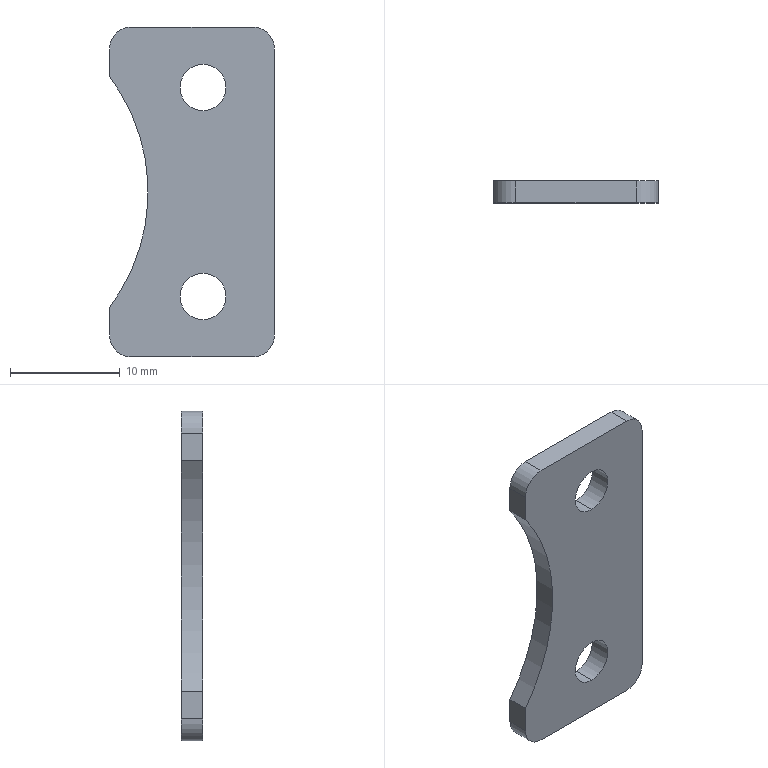Part | STEP file | 1 solid | 16 faces | box 15 x 2 x 30 mm | volume 737.571 mm3 | cylinder 9 | plane 7 | commonest cylinder face diameters 4 x4 4.2 x4 35 x1
STEP:
#1=CARTESIAN_POINT('',(0.,0.,0.));
#2=DIRECTION('',(0.,0.,1.));
#3=DIRECTION('',(1.,0.,0.));
#4=AXIS2_PLACEMENT_3D('',#1,#2,#3);
#5=CARTESIAN_POINT('',(1.,2.,7.4));
#6=VERTEX_POINT('',#5);
#7=CARTESIAN_POINT('',(1.,0.,7.4));
#8=VERTEX_POINT('',#7);
#9=CARTESIAN_POINT('',(1.,0.,7.4));
#10=DIRECTION('',(0.,-1.,0.));
#11=VECTOR('',#10,1.);
#12=LINE('',#9,#11);
#13=CARTESIAN_POINT('',(1.,0.,9.5));
#14=DIRECTION('',(0.,-1.,0.));
#15=DIRECTION('',(0.,0.,-1.));
#16=AXIS2_PLACEMENT_3D('',#13,#14,#15);
#17=CYLINDRICAL_SURFACE('',#16,2.1);
#18=CARTESIAN_POINT('',(6.283,0.));
#19=DIRECTION('',(0.,1.));
#20=VECTOR('',#19,1.);
#21=LINE('',#18,#20);
#22=(GEOMETRIC_REPRESENTATION_CONTEXT(2)PARAMETRIC_REPRESENTATION_CONTEXT()REPRESENTATION_CONTEXT('',''));
#23=DEFINITIONAL_REPRESENTATION('',(#21),#22);
#24=PCURVE('',#17,#23);
#25=CARTESIAN_POINT('',(1.,0.,9.5));
#26=DIRECTION('',(0.,-1.,0.));
#27=DIRECTION('',(0.,0.,-1.));
#28=AXIS2_PLACEMENT_3D('',#25,#26,#27);
#29=CYLINDRICAL_SURFACE('',#28,2.1);
#30=CARTESIAN_POINT('',(0.,0.));
#31=DIRECTION('',(0.,1.));
#32=VECTOR('',#31,1.);
#33=LINE('',#30,#32);
#34=(GEOMETRIC_REPRESENTATION_CONTEXT(2)PARAMETRIC_REPRESENTATION_CONTEXT()REPRESENTATION_CONTEXT('',''));
#35=DEFINITIONAL_REPRESENTATION('',(#33),#34);
#36=PCURVE('',#29,#35);
#37=SURFACE_CURVE('',#12,(#24,#36),.PCURVE_S1.);
#38=EDGE_CURVE('',#6,#8,#37,.T.);
#39=ORIENTED_EDGE('',*,*,#38,.T.);
#40=CARTESIAN_POINT('',(1.,0.,11.6));
#41=VERTEX_POINT('',#40);
#42=CARTESIAN_POINT('',(1.,0.,9.5));
#43=DIRECTION('',(0.,-1.,0.));
#44=DIRECTION('',(0.,0.,-1.));
#45=AXIS2_PLACEMENT_3D('',#42,#43,#44);
#46=CIRCLE('',#45,2.1);
#47=CARTESIAN_POINT('',(0.,0.));
#48=DIRECTION('',(1.,0.));
#49=VECTOR('',#48,1.);
#50=LINE('',#47,#49);
#51=(GEOMETRIC_REPRESENTATION_CONTEXT(2)PARAMETRIC_REPRESENTATION_CONTEXT()REPRESENTATION_CONTEXT('',''));
#52=DEFINITIONAL_REPRESENTATION('',(#50),#51);
#53=PCURVE('',#17,#52);
#54=CARTESIAN_POINT('',(0.,0.,0.));
#55=DIRECTION('',(0.,1.,0.));
#56=DIRECTION('',(0.,0.,1.));
#57=AXIS2_PLACEMENT_3D('',#54,#55,#56);
#58=PLANE('',#57);
#59=CARTESIAN_POINT('',(7.4,1.));
#60=CARTESIAN_POINT('',(7.4,4.637));
#61=CARTESIAN_POINT('',(10.55,2.819));
#62=CARTESIAN_POINT('',(13.7,1.));
#63=CARTESIAN_POINT('',(10.55,-0.8187));
#64=CARTESIAN_POINT('',(7.4,-2.637));
#65=CARTESIAN_POINT('',(7.4,1.));
#66=(BOUNDED_CURVE()B_SPLINE_CURVE(2,(#59,#60,#61,#62,#63,#64,#65),.UNSPECIFIED.,.T.,.F.)B_SPLINE_CURVE_WITH_KNOTS((1,2,2,2,2,1),(-2.094,0.,2.094,4.189,6.283,8.378),.UNSPECIFIED.)CURVE()GEOMETRIC_REPRESENTATION_ITEM()RATIONAL_B_SPLINE_CURVE((1.,0.5,1.,0.5,1.,0.5,1.))REPRESENTATION_ITEM(''));
#67=(GEOMETRIC_REPRESENTATION_CONTEXT(2)PARAMETRIC_REPRESENTATION_CONTEXT()REPRESENTATION_CONTEXT('',''));
#68=DEFINITIONAL_REPRESENTATION('',(#66),#67);
#69=PCURVE('',#58,#68);
#70=SURFACE_CURVE('',#46,(#53,#69),.PCURVE_S1.);
#71=EDGE_CURVE('',#41,#8,#70,.T.);
#72=ORIENTED_EDGE('',*,*,#71,.F.);
#73=CARTESIAN_POINT('',(1.,2.,11.6));
#74=VERTEX_POINT('',#73);
#75=CARTESIAN_POINT('',(1.,0.,11.6));
#76=DIRECTION('',(0.,-1.,0.));
#77=VECTOR('',#76,1.);
#78=LINE('',#75,#77);
#79=CARTESIAN_POINT('',(3.142,0.));
#80=DIRECTION('',(0.,1.));
#81=VECTOR('',#80,1.);
#82=LINE('',#79,#81);
#83=(GEOMETRIC_REPRESENTATION_CONTEXT(2)PARAMETRIC_REPRESENTATION_CONTEXT()REPRESENTATION_CONTEXT('',''));
#84=DEFINITIONAL_REPRESENTATION('',(#82),#83);
#85=PCURVE('',#17,#84);
#86=CARTESIAN_POINT('',(3.142,0.));
#87=DIRECTION('',(0.,1.));
#88=VECTOR('',#87,1.);
#89=LINE('',#86,#88);
#90=(GEOMETRIC_REPRESENTATION_CONTEXT(2)PARAMETRIC_REPRESENTATION_CONTEXT()REPRESENTATION_CONTEXT('',''));
#91=DEFINITIONAL_REPRESENTATION('',(#89),#90);
#92=PCURVE('',#29,#91);
#93=SURFACE_CURVE('',#78,(#85,#92),.PCURVE_S1.);
#94=EDGE_CURVE('',#74,#41,#93,.T.);
#95=ORIENTED_EDGE('',*,*,#94,.F.);
#96=CARTESIAN_POINT('',(1.,2.,9.5));
#97=DIRECTION('',(0.,-1.,0.));
#98=DIRECTION('',(0.,0.,-1.));
#99=AXIS2_PLACEMENT_3D('',#96,#97,#98);
#100=CIRCLE('',#99,2.1);
#101=CARTESIAN_POINT('',(0.,-2.));
#102=DIRECTION('',(1.,0.));
#103=VECTOR('',#102,1.);
#104=LINE('',#101,#103);
#105=(GEOMETRIC_REPRESENTATION_CONTEXT(2)PARAMETRIC_REPRESENTATION_CONTEXT()REPRESENTATION_CONTEXT('',''));
#106=DEFINITIONAL_REPRESENTATION('',(#104),#105);
#107=PCURVE('',#17,#106);
#108=CARTESIAN_POINT('',(0.,2.,0.));
#109=DIRECTION('',(0.,1.,0.));
#110=DIRECTION('',(0.,0.,1.));
#111=AXIS2_PLACEMENT_3D('',#108,#109,#110);
#112=PLANE('',#111);
#113=CARTESIAN_POINT('',(7.4,1.));
#114=CARTESIAN_POINT('',(7.4,4.637));
#115=CARTESIAN_POINT('',(10.55,2.819));
#116=CARTESIAN_POINT('',(13.7,1.));
#117=CARTESIAN_POINT('',(10.55,-0.8187));
#118=CARTESIAN_POINT('',(7.4,-2.637));
#119=CARTESIAN_POINT('',(7.4,1.));
#120=(BOUNDED_CURVE()B_SPLINE_CURVE(2,(#113,#114,#115,#116,#117,#118,#119),.UNSPECIFIED.,.T.,.F.)B_SPLINE_CURVE_WITH_KNOTS((1,2,2,2,2,1),(-2.094,0.,2.094,4.189,6.283,8.378),.UNSPECIFIED.)CURVE()GEOMETRIC_REPRESENTATION_ITEM()RATIONAL_B_SPLINE_CURVE((1.,0.5,1.,0.5,1.,0.5,1.))REPRESENTATION_ITEM(''));
#121=(GEOMETRIC_REPRESENTATION_CONTEXT(2)PARAMETRIC_REPRESENTATION_CONTEXT()REPRESENTATION_CONTEXT('',''));
#122=DEFINITIONAL_REPRESENTATION('',(#120),#121);
#123=PCURVE('',#112,#122);
#124=SURFACE_CURVE('',#100,(#107,#123),.PCURVE_S1.);
#125=EDGE_CURVE('',#74,#6,#124,.T.);
#126=ORIENTED_EDGE('',*,*,#125,.T.);
#127=EDGE_LOOP('',(#39,#72,#95,#126));
#128=FACE_BOUND('',#127,.F.);
#129=ADVANCED_FACE('',(#128),#17,.F.);
#130=CARTESIAN_POINT('',(1.,2.,-11.6));
#131=VERTEX_POINT('',#130);
#132=CARTESIAN_POINT('',(1.,0.,-11.6));
#133=VERTEX_POINT('',#132);
#134=CARTESIAN_POINT('',(1.,0.,-11.6));
#135=DIRECTION('',(0.,-1.,0.));
#136=VECTOR('',#135,1.);
#137=LINE('',#134,#136);
#138=CARTESIAN_POINT('',(1.,0.,-9.5));
#139=DIRECTION('',(0.,-1.,0.));
#140=DIRECTION('',(0.,0.,-1.));
#141=AXIS2_PLACEMENT_3D('',#138,#139,#140);
#142=CYLINDRICAL_SURFACE('',#141,2.1);
#143=CARTESIAN_POINT('',(6.283,0.));
#144=DIRECTION('',(0.,1.));
#145=VECTOR('',#144,1.);
#146=LINE('',#143,#145);
#147=(GEOMETRIC_REPRESENTATION_CONTEXT(2)PARAMETRIC_REPRESENTATION_CONTEXT()REPRESENTATION_CONTEXT('',''));
#148=DEFINITIONAL_REPRESENTATION('',(#146),#147);
#149=PCURVE('',#142,#148);
#150=CARTESIAN_POINT('',(1.,0.,-9.5));
#151=DIRECTION('',(0.,-1.,0.));
#152=DIRECTION('',(0.,0.,-1.));
#153=AXIS2_PLACEMENT_3D('',#150,#151,#152);
#154=CYLINDRICAL_SURFACE('',#153,2.1);
#155=CARTESIAN_POINT('',(0.,0.));
#156=DIRECTION('',(0.,1.));
#157=VECTOR('',#156,1.);
#158=LINE('',#155,#157);
#159=(GEOMETRIC_REPRESENTATION_CONTEXT(2)PARAMETRIC_REPRESENTATION_CONTEXT()REPRESENTATION_CONTEXT('',''));
#160=DEFINITIONAL_REPRESENTATION('',(#158),#159);
#161=PCURVE('',#154,#160);
#162=SURFACE_CURVE('',#137,(#149,#161),.PCURVE_S1.);
#163=EDGE_CURVE('',#131,#133,#162,.T.);
#164=ORIENTED_EDGE('',*,*,#163,.T.);
#165=CARTESIAN_POINT('',(1.,0.,-7.4));
#166=VERTEX_POINT('',#165);
#167=CARTESIAN_POINT('',(1.,0.,-9.5));
#168=DIRECTION('',(0.,-1.,0.));
#169=DIRECTION('',(0.,0.,-1.));
#170=AXIS2_PLACEMENT_3D('',#167,#168,#169);
#171=CIRCLE('',#170,2.1);
#172=CARTESIAN_POINT('',(0.,0.));
#173=DIRECTION('',(1.,0.));
#174=VECTOR('',#173,1.);
#175=LINE('',#172,#174);
#176=(GEOMETRIC_REPRESENTATION_CONTEXT(2)PARAMETRIC_REPRESENTATION_CONTEXT()REPRESENTATION_CONTEXT('',''));
#177=DEFINITIONAL_REPRESENTATION('',(#175),#176);
#178=PCURVE('',#142,#177);
#179=CARTESIAN_POINT('',(-11.6,1.));
#180=CARTESIAN_POINT('',(-11.6,4.637));
#181=CARTESIAN_POINT('',(-8.45,2.819));
#182=CARTESIAN_POINT('',(-5.3,1.));
#183=CARTESIAN_POINT('',(-8.45,-0.8187));
#184=CARTESIAN_POINT('',(-11.6,-2.637));
#185=CARTESIAN_POINT('',(-11.6,1.));
#186=(BOUNDED_CURVE()B_SPLINE_CURVE(2,(#179,#180,#181,#182,#183,#184,#185),.UNSPECIFIED.,.T.,.F.)B_SPLINE_CURVE_WITH_KNOTS((1,2,2,2,2,1),(-2.094,0.,2.094,4.189,6.283,8.378),.UNSPECIFIED.)CURVE()GEOMETRIC_REPRESENTATION_ITEM()RATIONAL_B_SPLINE_CURVE((1.,0.5,1.,0.5,1.,0.5,1.))REPRESENTATION_ITEM(''));
#187=(GEOMETRIC_REPRESENTATION_CONTEXT(2)PARAMETRIC_REPRESENTATION_CONTEXT()REPRESENTATION_CONTEXT('',''));
#188=DEFINITIONAL_REPRESENTATION('',(#186),#187);
#189=PCURVE('',#58,#188);
#190=SURFACE_CURVE('',#171,(#178,#189),.PCURVE_S1.);
#191=EDGE_CURVE('',#166,#133,#190,.T.);
#192=ORIENTED_EDGE('',*,*,#191,.F.);
#193=CARTESIAN_POINT('',(1.,2.,-7.4));
#194=VERTEX_POINT('',#193);
#195=CARTESIAN_POINT('',(1.,0.,-7.4));
#196=DIRECTION('',(0.,-1.,0.));
#197=VECTOR('',#196,1.);
#198=LINE('',#195,#197);
#199=CARTESIAN_POINT('',(3.142,0.));
#200=DIRECTION('',(0.,1.));
#201=VECTOR('',#200,1.);
#202=LINE('',#199,#201);
#203=(GEOMETRIC_REPRESENTATION_CONTEXT(2)PARAMETRIC_REPRESENTATION_CONTEXT()REPRESENTATION_CONTEXT('',''));
#204=DEFINITIONAL_REPRESENTATION('',(#202),#203);
#205=PCURVE('',#142,#204);
#206=CARTESIAN_POINT('',(3.142,0.));
#207=DIRECTION('',(0.,1.));
#208=VECTOR('',#207,1.);
#209=LINE('',#206,#208);
#210=(GEOMETRIC_REPRESENTATION_CONTEXT(2)PARAMETRIC_REPRESENTATION_CONTEXT()REPRESENTATION_CONTEXT('',''));
#211=DEFINITIONAL_REPRESENTATION('',(#209),#210);
#212=PCURVE('',#154,#211);
#213=SURFACE_CURVE('',#198,(#205,#212),.PCURVE_S1.);
#214=EDGE_CURVE('',#194,#166,#213,.T.);
#215=ORIENTED_EDGE('',*,*,#214,.F.);
#216=CARTESIAN_POINT('',(1.,2.,-9.5));
#217=DIRECTION('',(0.,-1.,0.));
#218=DIRECTION('',(0.,0.,-1.));
#219=AXIS2_PLACEMENT_3D('',#216,#217,#218);
#220=CIRCLE('',#219,2.1);
#221=CARTESIAN_POINT('',(0.,-2.));
#222=DIRECTION('',(1.,0.));
#223=VECTOR('',#222,1.);
#224=LINE('',#221,#223);
#225=(GEOMETRIC_REPRESENTATION_CONTEXT(2)PARAMETRIC_REPRESENTATION_CONTEXT()REPRESENTATION_CONTEXT('',''));
#226=DEFINITIONAL_REPRESENTATION('',(#224),#225);
#227=PCURVE('',#142,#226);
#228=CARTESIAN_POINT('',(-11.6,1.));
#229=CARTESIAN_POINT('',(-11.6,4.637));
#230=CARTESIAN_POINT('',(-8.45,2.819));
#231=CARTESIAN_POINT('',(-5.3,1.));
#232=CARTESIAN_POINT('',(-8.45,-0.8187));
#233=CARTESIAN_POINT('',(-11.6,-2.637));
#234=CARTESIAN_POINT('',(-11.6,1.));
#235=(BOUNDED_CURVE()B_SPLINE_CURVE(2,(#228,#229,#230,#231,#232,#233,#234),.UNSPECIFIED.,.T.,.F.)B_SPLINE_CURVE_WITH_KNOTS((1,2,2,2,2,1),(-2.094,0.,2.094,4.189,6.283,8.378),.UNSPECIFIED.)CURVE()GEOMETRIC_REPRESENTATION_ITEM()RATIONAL_B_SPLINE_CURVE((1.,0.5,1.,0.5,1.,0.5,1.))REPRESENTATION_ITEM(''));
#236=(GEOMETRIC_REPRESENTATION_CONTEXT(2)PARAMETRIC_REPRESENTATION_CONTEXT()REPRESENTATION_CONTEXT('',''));
#237=DEFINITIONAL_REPRESENTATION('',(#235),#236);
#238=PCURVE('',#112,#237);
#239=SURFACE_CURVE('',#220,(#227,#238),.PCURVE_S1.);
#240=EDGE_CURVE('',#194,#131,#239,.T.);
#241=ORIENTED_EDGE('',*,*,#240,.T.);
#242=EDGE_LOOP('',(#164,#192,#215,#241));
#243=FACE_BOUND('',#242,.F.);
#244=ADVANCED_FACE('',(#243),#142,.F.);
#245=CARTESIAN_POINT('',(-7.5,2.,-13.));
#246=VERTEX_POINT('',#245);
#247=CARTESIAN_POINT('',(-7.5,2.,-10.5));
#248=VERTEX_POINT('',#247);
#249=CARTESIAN_POINT('',(-7.5,2.,15.));
#250=DIRECTION('',(0.,0.,1.));
#251=VECTOR('',#250,1.);
#252=LINE('',#249,#251);
#253=CARTESIAN_POINT('',(-7.5,2.,15.));
#254=DIRECTION('',(1.,0.,0.));
#255=DIRECTION('',(0.,0.,-1.));
#256=AXIS2_PLACEMENT_3D('',#253,#254,#255);
#257=PLANE('',#256);
#258=CARTESIAN_POINT('',(0.,0.));
#259=DIRECTION('',(-1.,0.));
#260=VECTOR('',#259,1.);
#261=LINE('',#258,#260);
#262=(GEOMETRIC_REPRESENTATION_CONTEXT(2)PARAMETRIC_REPRESENTATION_CONTEXT()REPRESENTATION_CONTEXT('',''));
#263=DEFINITIONAL_REPRESENTATION('',(#261),#262);
#264=PCURVE('',#257,#263);
#265=CARTESIAN_POINT('',(15.,-7.5));
#266=DIRECTION('',(1.,0.));
#267=VECTOR('',#266,1.);
#268=LINE('',#265,#267);
#269=(GEOMETRIC_REPRESENTATION_CONTEXT(2)PARAMETRIC_REPRESENTATION_CONTEXT()REPRESENTATION_CONTEXT('',''));
#270=DEFINITIONAL_REPRESENTATION('',(#268),#269);
#271=PCURVE('',#112,#270);
#272=SURFACE_CURVE('',#252,(#264,#271),.PCURVE_S1.);
#273=EDGE_CURVE('',#246,#248,#272,.T.);
#274=ORIENTED_EDGE('',*,*,#273,.F.);
#275=CARTESIAN_POINT('',(-7.5,0.,-13.));
#276=VERTEX_POINT('',#275);
#277=CARTESIAN_POINT('',(-7.5,2.,-13.));
#278=DIRECTION('',(0.,-1.,0.));
#279=VECTOR('',#278,1.);
#280=LINE('',#277,#279);
#281=CARTESIAN_POINT('',(28.,0.));
#282=DIRECTION('',(0.,-1.));
#283=VECTOR('',#282,1.);
#284=LINE('',#281,#283);
#285=(GEOMETRIC_REPRESENTATION_CONTEXT(2)PARAMETRIC_REPRESENTATION_CONTEXT()REPRESENTATION_CONTEXT('',''));
#286=DEFINITIONAL_REPRESENTATION('',(#284),#285);
#287=PCURVE('',#257,#286);
#288=CARTESIAN_POINT('',(-5.5,2.,-13.));
#289=DIRECTION('',(0.,-1.,0.));
#290=DIRECTION('',(0.,0.,-1.));
#291=AXIS2_PLACEMENT_3D('',#288,#289,#290);
#292=CYLINDRICAL_SURFACE('',#291,2.);
#293=CARTESIAN_POINT('',(4.712,0.));
#294=DIRECTION('',(0.,1.));
#295=VECTOR('',#294,1.);
#296=LINE('',#293,#295);
#297=(GEOMETRIC_REPRESENTATION_CONTEXT(2)PARAMETRIC_REPRESENTATION_CONTEXT()REPRESENTATION_CONTEXT('',''));
#298=DEFINITIONAL_REPRESENTATION('',(#296),#297);
#299=PCURVE('',#292,#298);
#300=SURFACE_CURVE('',#280,(#287,#299),.PCURVE_S1.);
#301=EDGE_CURVE('',#246,#276,#300,.T.);
#302=ORIENTED_EDGE('',*,*,#301,.T.);
#303=CARTESIAN_POINT('',(-7.5,0.,-10.5));
#304=VERTEX_POINT('',#303);
#305=CARTESIAN_POINT('',(-7.5,0.,15.));
#306=DIRECTION('',(0.,0.,1.));
#307=VECTOR('',#306,1.);
#308=LINE('',#305,#307);
#309=CARTESIAN_POINT('',(0.,-2.));
#310=DIRECTION('',(-1.,0.));
#311=VECTOR('',#310,1.);
#312=LINE('',#309,#311);
#313=(GEOMETRIC_REPRESENTATION_CONTEXT(2)PARAMETRIC_REPRESENTATION_CONTEXT()REPRESENTATION_CONTEXT('',''));
#314=DEFINITIONAL_REPRESENTATION('',(#312),#313);
#315=PCURVE('',#257,#314);
#316=CARTESIAN_POINT('',(15.,-7.5));
#317=DIRECTION('',(1.,0.));
#318=VECTOR('',#317,1.);
#319=LINE('',#316,#318);
#320=(GEOMETRIC_REPRESENTATION_CONTEXT(2)PARAMETRIC_REPRESENTATION_CONTEXT()REPRESENTATION_CONTEXT('',''));
#321=DEFINITIONAL_REPRESENTATION('',(#319),#320);
#322=PCURVE('',#58,#321);
#323=SURFACE_CURVE('',#308,(#315,#322),.PCURVE_S1.);
#324=EDGE_CURVE('',#276,#304,#323,.T.);
#325=ORIENTED_EDGE('',*,*,#324,.T.);
#326=CARTESIAN_POINT('',(-7.5,0.,-10.5));
#327=DIRECTION('',(0.,1.,0.));
#328=VECTOR('',#327,1.);
#329=LINE('',#326,#328);
#330=CARTESIAN_POINT('',(25.5,-2.));
#331=DIRECTION('',(0.,1.));
#332=VECTOR('',#331,1.);
#333=LINE('',#330,#332);
#334=(GEOMETRIC_REPRESENTATION_CONTEXT(2)PARAMETRIC_REPRESENTATION_CONTEXT()REPRESENTATION_CONTEXT('',''));
#335=DEFINITIONAL_REPRESENTATION('',(#333),#334);
#336=PCURVE('',#257,#335);
#337=CARTESIAN_POINT('',(-21.5,0.,0.));
#338=DIRECTION('',(0.,1.,0.));
#339=DIRECTION('',(0.,0.,1.));
#340=AXIS2_PLACEMENT_3D('',#337,#338,#339);
#341=CYLINDRICAL_SURFACE('',#340,17.5);
#342=CARTESIAN_POINT('',(2.214,0.));
#343=DIRECTION('',(0.,1.));
#344=VECTOR('',#343,1.);
#345=LINE('',#342,#344);
#346=(GEOMETRIC_REPRESENTATION_CONTEXT(2)PARAMETRIC_REPRESENTATION_CONTEXT()REPRESENTATION_CONTEXT('',''));
#347=DEFINITIONAL_REPRESENTATION('',(#345),#346);
#348=PCURVE('',#341,#347);
#349=SURFACE_CURVE('',#329,(#336,#348),.PCURVE_S1.);
#350=EDGE_CURVE('',#304,#248,#349,.T.);
#351=ORIENTED_EDGE('',*,*,#350,.T.);
#352=EDGE_LOOP('',(#274,#302,#325,#351));
#353=FACE_BOUND('',#352,.T.);
#354=ADVANCED_FACE('',(#353),#257,.F.);
#355=CARTESIAN_POINT('',(-7.5,0.,10.5));
#356=VERTEX_POINT('',#355);
#357=CARTESIAN_POINT('',(-7.5,0.,13.));
#358=VERTEX_POINT('',#357);
#359=CARTESIAN_POINT('',(-7.5,0.,15.));
#360=DIRECTION('',(0.,0.,1.));
#361=VECTOR('',#360,1.);
#362=LINE('',#359,#361);
#363=CARTESIAN_POINT('',(-7.5,2.,15.));
#364=DIRECTION('',(1.,0.,0.));
#365=DIRECTION('',(0.,0.,-1.));
#366=AXIS2_PLACEMENT_3D('',#363,#364,#365);
#367=PLANE('',#366);
#368=CARTESIAN_POINT('',(0.,-2.));
#369=DIRECTION('',(-1.,0.));
#370=VECTOR('',#369,1.);
#371=LINE('',#368,#370);
#372=(GEOMETRIC_REPRESENTATION_CONTEXT(2)PARAMETRIC_REPRESENTATION_CONTEXT()REPRESENTATION_CONTEXT('',''));
#373=DEFINITIONAL_REPRESENTATION('',(#371),#372);
#374=PCURVE('',#367,#373);
#375=CARTESIAN_POINT('',(15.,-7.5));
#376=DIRECTION('',(1.,0.));
#377=VECTOR('',#376,1.);
#378=LINE('',#375,#377);
#379=(GEOMETRIC_REPRESENTATION_CONTEXT(2)PARAMETRIC_REPRESENTATION_CONTEXT()REPRESENTATION_CONTEXT('',''));
#380=DEFINITIONAL_REPRESENTATION('',(#378),#379);
#381=PCURVE('',#58,#380);
#382=SURFACE_CURVE('',#362,(#374,#381),.PCURVE_S1.);
#383=EDGE_CURVE('',#356,#358,#382,.T.);
#384=ORIENTED_EDGE('',*,*,#383,.T.);
#385=CARTESIAN_POINT('',(-7.5,2.,13.));
#386=VERTEX_POINT('',#385);
#387=CARTESIAN_POINT('',(-7.5,2.,13.));
#388=DIRECTION('',(0.,1.,0.));
#389=VECTOR('',#388,1.);
#390=LINE('',#387,#389);
#391=CARTESIAN_POINT('',(2.,0.));
#392=DIRECTION('',(0.,1.));
#393=VECTOR('',#392,1.);
#394=LINE('',#391,#393);
#395=(GEOMETRIC_REPRESENTATION_CONTEXT(2)PARAMETRIC_REPRESENTATION_CONTEXT()REPRESENTATION_CONTEXT('',''));
#396=DEFINITIONAL_REPRESENTATION('',(#394),#395);
#397=PCURVE('',#367,#396);
#398=CARTESIAN_POINT('',(-5.5,2.,13.));
#399=DIRECTION('',(0.,-1.,0.));
#400=DIRECTION('',(0.,0.,-1.));
#401=AXIS2_PLACEMENT_3D('',#398,#399,#400);
#402=CYLINDRICAL_SURFACE('',#401,2.);
#403=CARTESIAN_POINT('',(4.712,0.));
#404=DIRECTION('',(0.,-1.));
#405=VECTOR('',#404,1.);
#406=LINE('',#403,#405);
#407=(GEOMETRIC_REPRESENTATION_CONTEXT(2)PARAMETRIC_REPRESENTATION_CONTEXT()REPRESENTATION_CONTEXT('',''));
#408=DEFINITIONAL_REPRESENTATION('',(#406),#407);
#409=PCURVE('',#402,#408);
#410=SURFACE_CURVE('',#390,(#397,#409),.PCURVE_S1.);
#411=EDGE_CURVE('',#358,#386,#410,.T.);
#412=ORIENTED_EDGE('',*,*,#411,.T.);
#413=CARTESIAN_POINT('',(-7.5,2.,10.5));
#414=VERTEX_POINT('',#413);
#415=CARTESIAN_POINT('',(-7.5,2.,15.));
#416=DIRECTION('',(0.,0.,1.));
#417=VECTOR('',#416,1.);
#418=LINE('',#415,#417);
#419=CARTESIAN_POINT('',(0.,0.));
#420=DIRECTION('',(-1.,0.));
#421=VECTOR('',#420,1.);
#422=LINE('',#419,#421);
#423=(GEOMETRIC_REPRESENTATION_CONTEXT(2)PARAMETRIC_REPRESENTATION_CONTEXT()REPRESENTATION_CONTEXT('',''));
#424=DEFINITIONAL_REPRESENTATION('',(#422),#423);
#425=PCURVE('',#367,#424);
#426=CARTESIAN_POINT('',(15.,-7.5));
#427=DIRECTION('',(1.,0.));
#428=VECTOR('',#427,1.);
#429=LINE('',#426,#428);
#430=(GEOMETRIC_REPRESENTATION_CONTEXT(2)PARAMETRIC_REPRESENTATION_CONTEXT()REPRESENTATION_CONTEXT('',''));
#431=DEFINITIONAL_REPRESENTATION('',(#429),#430);
#432=PCURVE('',#112,#431);
#433=SURFACE_CURVE('',#418,(#425,#432),.PCURVE_S1.);
#434=EDGE_CURVE('',#414,#386,#433,.T.);
#435=ORIENTED_EDGE('',*,*,#434,.F.);
#436=CARTESIAN_POINT('',(-7.5,0.,10.5));
#437=DIRECTION('',(0.,-1.,0.));
#438=VECTOR('',#437,1.);
#439=LINE('',#436,#438);
#440=CARTESIAN_POINT('',(4.5,-2.));
#441=DIRECTION('',(0.,-1.));
#442=VECTOR('',#441,1.);
#443=LINE('',#440,#442);
#444=(GEOMETRIC_REPRESENTATION_CONTEXT(2)PARAMETRIC_REPRESENTATION_CONTEXT()REPRESENTATION_CONTEXT('',''));
#445=DEFINITIONAL_REPRESENTATION('',(#443),#444);
#446=PCURVE('',#367,#445);
#447=CARTESIAN_POINT('',(0.9273,0.));
#448=DIRECTION('',(0.,-1.));
#449=VECTOR('',#448,1.);
#450=LINE('',#447,#449);
#451=(GEOMETRIC_REPRESENTATION_CONTEXT(2)PARAMETRIC_REPRESENTATION_CONTEXT()REPRESENTATION_CONTEXT('',''));
#452=DEFINITIONAL_REPRESENTATION('',(#450),#451);
#453=PCURVE('',#341,#452);
#454=SURFACE_CURVE('',#439,(#446,#453),.PCURVE_S1.);
#455=EDGE_CURVE('',#414,#356,#454,.T.);
#456=ORIENTED_EDGE('',*,*,#455,.T.);
#457=EDGE_LOOP('',(#384,#412,#435,#456));
#458=FACE_BOUND('',#457,.T.);
#459=ADVANCED_FACE('',(#458),#367,.F.);
#460=CARTESIAN_POINT('',(-5.5,2.,15.));
#461=VERTEX_POINT('',#460);
#462=CARTESIAN_POINT('',(5.5,2.,15.));
#463=VERTEX_POINT('',#462);
#464=CARTESIAN_POINT('',(7.5,2.,15.));
#465=DIRECTION('',(1.,0.,0.));
#466=VECTOR('',#465,1.);
#467=LINE('',#464,#466);
#468=CARTESIAN_POINT('',(7.5,2.,15.));
#469=DIRECTION('',(0.,0.,-1.));
#470=DIRECTION('',(-1.,0.,0.));
#471=AXIS2_PLACEMENT_3D('',#468,#469,#470);
#472=PLANE('',#471);
#473=CARTESIAN_POINT('',(0.,0.));
#474=DIRECTION('',(-1.,0.));
#475=VECTOR('',#474,1.);
#476=LINE('',#473,#475);
#477=(GEOMETRIC_REPRESENTATION_CONTEXT(2)PARAMETRIC_REPRESENTATION_CONTEXT()REPRESENTATION_CONTEXT('',''));
#478=DEFINITIONAL_REPRESENTATION('',(#476),#477);
#479=PCURVE('',#472,#478);
#480=CARTESIAN_POINT('',(15.,7.5));
#481=DIRECTION('',(0.,1.));
#482=VECTOR('',#481,1.);
#483=LINE('',#480,#482);
#484=(GEOMETRIC_REPRESENTATION_CONTEXT(2)PARAMETRIC_REPRESENTATION_CONTEXT()REPRESENTATION_CONTEXT('',''));
#485=DEFINITIONAL_REPRESENTATION('',(#483),#484);
#486=PCURVE('',#112,#485);
#487=SURFACE_CURVE('',#467,(#479,#486),.PCURVE_S1.);
#488=EDGE_CURVE('',#461,#463,#487,.T.);
#489=ORIENTED_EDGE('',*,*,#488,.F.);
#490=CARTESIAN_POINT('',(-5.5,0.,15.));
#491=VERTEX_POINT('',#490);
#492=CARTESIAN_POINT('',(-5.5,2.,15.));
#493=DIRECTION('',(0.,-1.,0.));
#494=VECTOR('',#493,1.);
#495=LINE('',#492,#494);
#496=CARTESIAN_POINT('',(13.,0.));
#497=DIRECTION('',(0.,-1.));
#498=VECTOR('',#497,1.);
#499=LINE('',#496,#498);
#500=(GEOMETRIC_REPRESENTATION_CONTEXT(2)PARAMETRIC_REPRESENTATION_CONTEXT()REPRESENTATION_CONTEXT('',''));
#501=DEFINITIONAL_REPRESENTATION('',(#499),#500);
#502=PCURVE('',#472,#501);
#503=CARTESIAN_POINT('',(3.142,0.));
#504=DIRECTION('',(0.,1.));
#505=VECTOR('',#504,1.);
#506=LINE('',#503,#505);
#507=(GEOMETRIC_REPRESENTATION_CONTEXT(2)PARAMETRIC_REPRESENTATION_CONTEXT()REPRESENTATION_CONTEXT('',''));
#508=DEFINITIONAL_REPRESENTATION('',(#506),#507);
#509=PCURVE('',#402,#508);
#510=SURFACE_CURVE('',#495,(#502,#509),.PCURVE_S1.);
#511=EDGE_CURVE('',#461,#491,#510,.T.);
#512=ORIENTED_EDGE('',*,*,#511,.T.);
#513=CARTESIAN_POINT('',(5.5,0.,15.));
#514=VERTEX_POINT('',#513);
#515=CARTESIAN_POINT('',(7.5,0.,15.));
#516=DIRECTION('',(1.,0.,0.));
#517=VECTOR('',#516,1.);
#518=LINE('',#515,#517);
#519=CARTESIAN_POINT('',(0.,-2.));
#520=DIRECTION('',(-1.,0.));
#521=VECTOR('',#520,1.);
#522=LINE('',#519,#521);
#523=(GEOMETRIC_REPRESENTATION_CONTEXT(2)PARAMETRIC_REPRESENTATION_CONTEXT()REPRESENTATION_CONTEXT('',''));
#524=DEFINITIONAL_REPRESENTATION('',(#522),#523);
#525=PCURVE('',#472,#524);
#526=CARTESIAN_POINT('',(15.,7.5));
#527=DIRECTION('',(0.,1.));
#528=VECTOR('',#527,1.);
#529=LINE('',#526,#528);
#530=(GEOMETRIC_REPRESENTATION_CONTEXT(2)PARAMETRIC_REPRESENTATION_CONTEXT()REPRESENTATION_CONTEXT('',''));
#531=DEFINITIONAL_REPRESENTATION('',(#529),#530);
#532=PCURVE('',#58,#531);
#533=SURFACE_CURVE('',#518,(#525,#532),.PCURVE_S1.);
#534=EDGE_CURVE('',#491,#514,#533,.T.);
#535=ORIENTED_EDGE('',*,*,#534,.T.);
#536=CARTESIAN_POINT('',(5.5,2.,15.));
#537=DIRECTION('',(0.,1.,0.));
#538=VECTOR('',#537,1.);
#539=LINE('',#536,#538);
#540=CARTESIAN_POINT('',(2.,0.));
#541=DIRECTION('',(0.,1.));
#542=VECTOR('',#541,1.);
#543=LINE('',#540,#542);
#544=(GEOMETRIC_REPRESENTATION_CONTEXT(2)PARAMETRIC_REPRESENTATION_CONTEXT()REPRESENTATION_CONTEXT('',''));
#545=DEFINITIONAL_REPRESENTATION('',(#543),#544);
#546=PCURVE('',#472,#545);
#547=CARTESIAN_POINT('',(5.5,2.,13.));
#548=DIRECTION('',(0.,-1.,0.));
#549=DIRECTION('',(0.,0.,-1.));
#550=AXIS2_PLACEMENT_3D('',#547,#548,#549);
#551=CYLINDRICAL_SURFACE('',#550,2.);
#552=CARTESIAN_POINT('',(3.142,0.));
#553=DIRECTION('',(0.,-1.));
#554=VECTOR('',#553,1.);
#555=LINE('',#552,#554);
#556=(GEOMETRIC_REPRESENTATION_CONTEXT(2)PARAMETRIC_REPRESENTATION_CONTEXT()REPRESENTATION_CONTEXT('',''));
#557=DEFINITIONAL_REPRESENTATION('',(#555),#556);
#558=PCURVE('',#551,#557);
#559=SURFACE_CURVE('',#539,(#546,#558),.PCURVE_S1.);
#560=EDGE_CURVE('',#514,#463,#559,.T.);
#561=ORIENTED_EDGE('',*,*,#560,.T.);
#562=EDGE_LOOP('',(#489,#512,#535,#561));
#563=FACE_BOUND('',#562,.T.);
#564=ADVANCED_FACE('',(#563),#472,.F.);
#565=CARTESIAN_POINT('',(7.5,0.,13.));
#566=VERTEX_POINT('',#565);
#567=CARTESIAN_POINT('',(7.5,0.,-13.));
#568=VERTEX_POINT('',#567);
#569=CARTESIAN_POINT('',(7.5,0.,15.));
#570=DIRECTION('',(0.,0.,-1.));
#571=VECTOR('',#570,1.);
#572=LINE('',#569,#571);
#573=CARTESIAN_POINT('',(7.5,2.,15.));
#574=DIRECTION('',(-1.,0.,0.));
#575=DIRECTION('',(0.,0.,1.));
#576=AXIS2_PLACEMENT_3D('',#573,#574,#575);
#577=PLANE('',#576);
#578=CARTESIAN_POINT('',(0.,-2.));
#579=DIRECTION('',(-1.,0.));
#580=VECTOR('',#579,1.);
#581=LINE('',#578,#580);
#582=(GEOMETRIC_REPRESENTATION_CONTEXT(2)PARAMETRIC_REPRESENTATION_CONTEXT()REPRESENTATION_CONTEXT('',''));
#583=DEFINITIONAL_REPRESENTATION('',(#581),#582);
#584=PCURVE('',#577,#583);
#585=CARTESIAN_POINT('',(15.,7.5));
#586=DIRECTION('',(-1.,0.));
#587=VECTOR('',#586,1.);
#588=LINE('',#585,#587);
#589=(GEOMETRIC_REPRESENTATION_CONTEXT(2)PARAMETRIC_REPRESENTATION_CONTEXT()REPRESENTATION_CONTEXT('',''));
#590=DEFINITIONAL_REPRESENTATION('',(#588),#589);
#591=PCURVE('',#58,#590);
#592=SURFACE_CURVE('',#572,(#584,#591),.PCURVE_S1.);
#593=EDGE_CURVE('',#566,#568,#592,.T.);
#594=ORIENTED_EDGE('',*,*,#593,.T.);
#595=CARTESIAN_POINT('',(7.5,2.,-13.));
#596=VERTEX_POINT('',#595);
#597=CARTESIAN_POINT('',(7.5,2.,-13.));
#598=DIRECTION('',(0.,1.,0.));
#599=VECTOR('',#598,1.);
#600=LINE('',#597,#599);
#601=CARTESIAN_POINT('',(-28.,0.));
#602=DIRECTION('',(0.,1.));
#603=VECTOR('',#602,1.);
#604=LINE('',#601,#603);
#605=(GEOMETRIC_REPRESENTATION_CONTEXT(2)PARAMETRIC_REPRESENTATION_CONTEXT()REPRESENTATION_CONTEXT('',''));
#606=DEFINITIONAL_REPRESENTATION('',(#604),#605);
#607=PCURVE('',#577,#606);
#608=CARTESIAN_POINT('',(5.5,2.,-13.));
#609=DIRECTION('',(0.,-1.,0.));
#610=DIRECTION('',(0.,0.,-1.));
#611=AXIS2_PLACEMENT_3D('',#608,#609,#610);
#612=CYLINDRICAL_SURFACE('',#611,2.);
#613=CARTESIAN_POINT('',(1.571,0.));
#614=DIRECTION('',(0.,-1.));
#615=VECTOR('',#614,1.);
#616=LINE('',#613,#615);
#617=(GEOMETRIC_REPRESENTATION_CONTEXT(2)PARAMETRIC_REPRESENTATION_CONTEXT()REPRESENTATION_CONTEXT('',''));
#618=DEFINITIONAL_REPRESENTATION('',(#616),#617);
#619=PCURVE('',#612,#618);
#620=SURFACE_CURVE('',#600,(#607,#619),.PCURVE_S1.);
#621=EDGE_CURVE('',#568,#596,#620,.T.);
#622=ORIENTED_EDGE('',*,*,#621,.T.);
#623=CARTESIAN_POINT('',(7.5,2.,13.));
#624=VERTEX_POINT('',#623);
#625=CARTESIAN_POINT('',(7.5,2.,15.));
#626=DIRECTION('',(0.,0.,-1.));
#627=VECTOR('',#626,1.);
#628=LINE('',#625,#627);
#629=CARTESIAN_POINT('',(0.,0.));
#630=DIRECTION('',(-1.,0.));
#631=VECTOR('',#630,1.);
#632=LINE('',#629,#631);
#633=(GEOMETRIC_REPRESENTATION_CONTEXT(2)PARAMETRIC_REPRESENTATION_CONTEXT()REPRESENTATION_CONTEXT('',''));
#634=DEFINITIONAL_REPRESENTATION('',(#632),#633);
#635=PCURVE('',#577,#634);
#636=CARTESIAN_POINT('',(15.,7.5));
#637=DIRECTION('',(-1.,0.));
#638=VECTOR('',#637,1.);
#639=LINE('',#636,#638);
#640=(GEOMETRIC_REPRESENTATION_CONTEXT(2)PARAMETRIC_REPRESENTATION_CONTEXT()REPRESENTATION_CONTEXT('',''));
#641=DEFINITIONAL_REPRESENTATION('',(#639),#640);
#642=PCURVE('',#112,#641);
#643=SURFACE_CURVE('',#628,(#635,#642),.PCURVE_S1.);
#644=EDGE_CURVE('',#624,#596,#643,.T.);
#645=ORIENTED_EDGE('',*,*,#644,.F.);
#646=CARTESIAN_POINT('',(7.5,2.,13.));
#647=DIRECTION('',(0.,-1.,0.));
#648=VECTOR('',#647,1.);
#649=LINE('',#646,#648);
#650=CARTESIAN_POINT('',(-2.,0.));
#651=DIRECTION('',(0.,-1.));
#652=VECTOR('',#651,1.);
#653=LINE('',#650,#652);
#654=(GEOMETRIC_REPRESENTATION_CONTEXT(2)PARAMETRIC_REPRESENTATION_CONTEXT()REPRESENTATION_CONTEXT('',''));
#655=DEFINITIONAL_REPRESENTATION('',(#653),#654);
#656=PCURVE('',#577,#655);
#657=CARTESIAN_POINT('',(1.571,0.));
#658=DIRECTION('',(0.,1.));
#659=VECTOR('',#658,1.);
#660=LINE('',#657,#659);
#661=(GEOMETRIC_REPRESENTATION_CONTEXT(2)PARAMETRIC_REPRESENTATION_CONTEXT()REPRESENTATION_CONTEXT('',''));
#662=DEFINITIONAL_REPRESENTATION('',(#660),#661);
#663=PCURVE('',#551,#662);
#664=SURFACE_CURVE('',#649,(#656,#663),.PCURVE_S1.);
#665=EDGE_CURVE('',#624,#566,#664,.T.);
#666=ORIENTED_EDGE('',*,*,#665,.T.);
#667=EDGE_LOOP('',(#594,#622,#645,#666));
#668=FACE_BOUND('',#667,.T.);
#669=ADVANCED_FACE('',(#668),#577,.F.);
#670=CARTESIAN_POINT('',(5.5,2.,-15.));
#671=VERTEX_POINT('',#670);
#672=CARTESIAN_POINT('',(-5.5,2.,-15.));
#673=VERTEX_POINT('',#672);
#674=CARTESIAN_POINT('',(7.5,2.,-15.));
#675=DIRECTION('',(-1.,0.,0.));
#676=VECTOR('',#675,1.);
#677=LINE('',#674,#676);
#678=CARTESIAN_POINT('',(7.5,2.,-15.));
#679=DIRECTION('',(0.,0.,1.));
#680=DIRECTION('',(1.,0.,0.));
#681=AXIS2_PLACEMENT_3D('',#678,#679,#680);
#682=PLANE('',#681);
#683=CARTESIAN_POINT('',(0.,0.));
#684=DIRECTION('',(-1.,0.));
#685=VECTOR('',#684,1.);
#686=LINE('',#683,#685);
#687=(GEOMETRIC_REPRESENTATION_CONTEXT(2)PARAMETRIC_REPRESENTATION_CONTEXT()REPRESENTATION_CONTEXT('',''));
#688=DEFINITIONAL_REPRESENTATION('',(#686),#687);
#689=PCURVE('',#682,#688);
#690=CARTESIAN_POINT('',(-15.,7.5));
#691=DIRECTION('',(0.,-1.));
#692=VECTOR('',#691,1.);
#693=LINE('',#690,#692);
#694=(GEOMETRIC_REPRESENTATION_CONTEXT(2)PARAMETRIC_REPRESENTATION_CONTEXT()REPRESENTATION_CONTEXT('',''));
#695=DEFINITIONAL_REPRESENTATION('',(#693),#694);
#696=PCURVE('',#112,#695);
#697=SURFACE_CURVE('',#677,(#689,#696),.PCURVE_S1.);
#698=EDGE_CURVE('',#671,#673,#697,.T.);
#699=ORIENTED_EDGE('',*,*,#698,.F.);
#700=CARTESIAN_POINT('',(5.5,0.,-15.));
#701=VERTEX_POINT('',#700);
#702=CARTESIAN_POINT('',(5.5,2.,-15.));
#703=DIRECTION('',(0.,-1.,0.));
#704=VECTOR('',#703,1.);
#705=LINE('',#702,#704);
#706=CARTESIAN_POINT('',(-2.,0.));
#707=DIRECTION('',(0.,-1.));
#708=VECTOR('',#707,1.);
#709=LINE('',#706,#708);
#710=(GEOMETRIC_REPRESENTATION_CONTEXT(2)PARAMETRIC_REPRESENTATION_CONTEXT()REPRESENTATION_CONTEXT('',''));
#711=DEFINITIONAL_REPRESENTATION('',(#709),#710);
#712=PCURVE('',#682,#711);
#713=CARTESIAN_POINT('',(0.,0.));
#714=DIRECTION('',(0.,1.));
#715=VECTOR('',#714,1.);
#716=LINE('',#713,#715);
#717=(GEOMETRIC_REPRESENTATION_CONTEXT(2)PARAMETRIC_REPRESENTATION_CONTEXT()REPRESENTATION_CONTEXT('',''));
#718=DEFINITIONAL_REPRESENTATION('',(#716),#717);
#719=PCURVE('',#612,#718);
#720=SURFACE_CURVE('',#705,(#712,#719),.PCURVE_S1.);
#721=EDGE_CURVE('',#671,#701,#720,.T.);
#722=ORIENTED_EDGE('',*,*,#721,.T.);
#723=CARTESIAN_POINT('',(-5.5,0.,-15.));
#724=VERTEX_POINT('',#723);
#725=CARTESIAN_POINT('',(7.5,0.,-15.));
#726=DIRECTION('',(-1.,0.,0.));
#727=VECTOR('',#726,1.);
#728=LINE('',#725,#727);
#729=CARTESIAN_POINT('',(0.,-2.));
#730=DIRECTION('',(-1.,0.));
#731=VECTOR('',#730,1.);
#732=LINE('',#729,#731);
#733=(GEOMETRIC_REPRESENTATION_CONTEXT(2)PARAMETRIC_REPRESENTATION_CONTEXT()REPRESENTATION_CONTEXT('',''));
#734=DEFINITIONAL_REPRESENTATION('',(#732),#733);
#735=PCURVE('',#682,#734);
#736=CARTESIAN_POINT('',(-15.,7.5));
#737=DIRECTION('',(0.,-1.));
#738=VECTOR('',#737,1.);
#739=LINE('',#736,#738);
#740=(GEOMETRIC_REPRESENTATION_CONTEXT(2)PARAMETRIC_REPRESENTATION_CONTEXT()REPRESENTATION_CONTEXT('',''));
#741=DEFINITIONAL_REPRESENTATION('',(#739),#740);
#742=PCURVE('',#58,#741);
#743=SURFACE_CURVE('',#728,(#735,#742),.PCURVE_S1.);
#744=EDGE_CURVE('',#701,#724,#743,.T.);
#745=ORIENTED_EDGE('',*,*,#744,.T.);
#746=CARTESIAN_POINT('',(-5.5,2.,-15.));
#747=DIRECTION('',(0.,1.,0.));
#748=VECTOR('',#747,1.);
#749=LINE('',#746,#748);
#750=CARTESIAN_POINT('',(-13.,0.));
#751=DIRECTION('',(0.,1.));
#752=VECTOR('',#751,1.);
#753=LINE('',#750,#752);
#754=(GEOMETRIC_REPRESENTATION_CONTEXT(2)PARAMETRIC_REPRESENTATION_CONTEXT()REPRESENTATION_CONTEXT('',''));
#755=DEFINITIONAL_REPRESENTATION('',(#753),#754);
#756=PCURVE('',#682,#755);
#757=CARTESIAN_POINT('',(6.283,0.));
#758=DIRECTION('',(0.,-1.));
#759=VECTOR('',#758,1.);
#760=LINE('',#757,#759);
#761=(GEOMETRIC_REPRESENTATION_CONTEXT(2)PARAMETRIC_REPRESENTATION_CONTEXT()REPRESENTATION_CONTEXT('',''));
#762=DEFINITIONAL_REPRESENTATION('',(#760),#761);
#763=PCURVE('',#292,#762);
#764=SURFACE_CURVE('',#749,(#756,#763),.PCURVE_S1.);
#765=EDGE_CURVE('',#724,#673,#764,.T.);
#766=ORIENTED_EDGE('',*,*,#765,.T.);
#767=EDGE_LOOP('',(#699,#722,#745,#766));
#768=FACE_BOUND('',#767,.T.);
#769=ADVANCED_FACE('',(#768),#682,.F.);
#770=CARTESIAN_POINT('',(1.,2.,9.5));
#771=DIRECTION('',(0.,-1.,0.));
#772=DIRECTION('',(0.,0.,-1.));
#773=AXIS2_PLACEMENT_3D('',#770,#771,#772);
#774=CIRCLE('',#773,2.1);
#775=CARTESIAN_POINT('',(7.4,1.));
#776=CARTESIAN_POINT('',(7.4,4.637));
#777=CARTESIAN_POINT('',(10.55,2.819));
#778=CARTESIAN_POINT('',(13.7,1.));
#779=CARTESIAN_POINT('',(10.55,-0.8187));
#780=CARTESIAN_POINT('',(7.4,-2.637));
#781=CARTESIAN_POINT('',(7.4,1.));
#782=(BOUNDED_CURVE()B_SPLINE_CURVE(2,(#775,#776,#777,#778,#779,#780,#781),.UNSPECIFIED.,.T.,.F.)B_SPLINE_CURVE_WITH_KNOTS((1,2,2,2,2,1),(-2.094,0.,2.094,4.189,6.283,8.378),.UNSPECIFIED.)CURVE()GEOMETRIC_REPRESENTATION_ITEM()RATIONAL_B_SPLINE_CURVE((1.,0.5,1.,0.5,1.,0.5,1.))REPRESENTATION_ITEM(''));
#783=(GEOMETRIC_REPRESENTATION_CONTEXT(2)PARAMETRIC_REPRESENTATION_CONTEXT()REPRESENTATION_CONTEXT('',''));
#784=DEFINITIONAL_REPRESENTATION('',(#782),#783);
#785=PCURVE('',#112,#784);
#786=CARTESIAN_POINT('',(0.,-2.));
#787=DIRECTION('',(1.,0.));
#788=VECTOR('',#787,1.);
#789=LINE('',#786,#788);
#790=(GEOMETRIC_REPRESENTATION_CONTEXT(2)PARAMETRIC_REPRESENTATION_CONTEXT()REPRESENTATION_CONTEXT('',''));
#791=DEFINITIONAL_REPRESENTATION('',(#789),#790);
#792=PCURVE('',#29,#791);
#793=SURFACE_CURVE('',#774,(#785,#792),.PCURVE_S1.);
#794=EDGE_CURVE('',#6,#74,#793,.T.);
#795=ORIENTED_EDGE('',*,*,#794,.T.);
#796=ORIENTED_EDGE('',*,*,#125,.T.);
#797=EDGE_LOOP('',(#795,#796));
#798=FACE_BOUND('',#797,.T.);
#799=CARTESIAN_POINT('',(1.,2.,-9.5));
#800=DIRECTION('',(0.,-1.,0.));
#801=DIRECTION('',(0.,0.,-1.));
#802=AXIS2_PLACEMENT_3D('',#799,#800,#801);
#803=CIRCLE('',#802,2.1);
#804=CARTESIAN_POINT('',(-11.6,1.));
#805=CARTESIAN_POINT('',(-11.6,4.637));
#806=CARTESIAN_POINT('',(-8.45,2.819));
#807=CARTESIAN_POINT('',(-5.3,1.));
#808=CARTESIAN_POINT('',(-8.45,-0.8187));
#809=CARTESIAN_POINT('',(-11.6,-2.637));
#810=CARTESIAN_POINT('',(-11.6,1.));
#811=(BOUNDED_CURVE()B_SPLINE_CURVE(2,(#804,#805,#806,#807,#808,#809,#810),.UNSPECIFIED.,.T.,.F.)B_SPLINE_CURVE_WITH_KNOTS((1,2,2,2,2,1),(-2.094,0.,2.094,4.189,6.283,8.378),.UNSPECIFIED.)CURVE()GEOMETRIC_REPRESENTATION_ITEM()RATIONAL_B_SPLINE_CURVE((1.,0.5,1.,0.5,1.,0.5,1.))REPRESENTATION_ITEM(''));
#812=(GEOMETRIC_REPRESENTATION_CONTEXT(2)PARAMETRIC_REPRESENTATION_CONTEXT()REPRESENTATION_CONTEXT('',''));
#813=DEFINITIONAL_REPRESENTATION('',(#811),#812);
#814=PCURVE('',#112,#813);
#815=CARTESIAN_POINT('',(0.,-2.));
#816=DIRECTION('',(1.,0.));
#817=VECTOR('',#816,1.);
#818=LINE('',#815,#817);
#819=(GEOMETRIC_REPRESENTATION_CONTEXT(2)PARAMETRIC_REPRESENTATION_CONTEXT()REPRESENTATION_CONTEXT('',''));
#820=DEFINITIONAL_REPRESENTATION('',(#818),#819);
#821=PCURVE('',#154,#820);
#822=SURFACE_CURVE('',#803,(#814,#821),.PCURVE_S1.);
#823=EDGE_CURVE('',#131,#194,#822,.T.);
#824=ORIENTED_EDGE('',*,*,#823,.T.);
#825=ORIENTED_EDGE('',*,*,#240,.T.);
#826=EDGE_LOOP('',(#824,#825));
#827=FACE_BOUND('',#826,.T.);
#828=ORIENTED_EDGE('',*,*,#644,.T.);
#829=CARTESIAN_POINT('',(5.5,2.,-13.));
#830=DIRECTION('',(0.,1.,0.));
#831=DIRECTION('',(0.,0.,1.));
#832=AXIS2_PLACEMENT_3D('',#829,#830,#831);
#833=CIRCLE('',#832,2.);
#834=CARTESIAN_POINT('',(-13.,5.5));
#835=DIRECTION('',(1.,0.));
#836=AXIS2_PLACEMENT_2D('',#834,#835);
#837=CIRCLE('',#836,2.);
#838=(GEOMETRIC_REPRESENTATION_CONTEXT(2)PARAMETRIC_REPRESENTATION_CONTEXT()REPRESENTATION_CONTEXT('',''));
#839=DEFINITIONAL_REPRESENTATION('',(#837),#838);
#840=PCURVE('',#112,#839);
#841=CARTESIAN_POINT('',(3.142,0.));
#842=DIRECTION('',(-1.,0.));
#843=VECTOR('',#842,1.);
#844=LINE('',#841,#843);
#845=(GEOMETRIC_REPRESENTATION_CONTEXT(2)PARAMETRIC_REPRESENTATION_CONTEXT()REPRESENTATION_CONTEXT('',''));
#846=DEFINITIONAL_REPRESENTATION('',(#844),#845);
#847=PCURVE('',#612,#846);
#848=SURFACE_CURVE('',#833,(#840,#847),.PCURVE_S1.);
#849=EDGE_CURVE('',#596,#671,#848,.T.);
#850=ORIENTED_EDGE('',*,*,#849,.T.);
#851=ORIENTED_EDGE('',*,*,#698,.T.);
#852=CARTESIAN_POINT('',(-5.5,2.,-13.));
#853=DIRECTION('',(0.,1.,0.));
#854=DIRECTION('',(0.,0.,1.));
#855=AXIS2_PLACEMENT_3D('',#852,#853,#854);
#856=CIRCLE('',#855,2.);
#857=CARTESIAN_POINT('',(-13.,-5.5));
#858=DIRECTION('',(1.,0.));
#859=AXIS2_PLACEMENT_2D('',#857,#858);
#860=CIRCLE('',#859,2.);
#861=(GEOMETRIC_REPRESENTATION_CONTEXT(2)PARAMETRIC_REPRESENTATION_CONTEXT()REPRESENTATION_CONTEXT('',''));
#862=DEFINITIONAL_REPRESENTATION('',(#860),#861);
#863=PCURVE('',#112,#862);
#864=CARTESIAN_POINT('',(9.425,0.));
#865=DIRECTION('',(-1.,0.));
#866=VECTOR('',#865,1.);
#867=LINE('',#864,#866);
#868=(GEOMETRIC_REPRESENTATION_CONTEXT(2)PARAMETRIC_REPRESENTATION_CONTEXT()REPRESENTATION_CONTEXT('',''));
#869=DEFINITIONAL_REPRESENTATION('',(#867),#868);
#870=PCURVE('',#292,#869);
#871=SURFACE_CURVE('',#856,(#863,#870),.PCURVE_S1.);
#872=EDGE_CURVE('',#673,#246,#871,.T.);
#873=ORIENTED_EDGE('',*,*,#872,.T.);
#874=ORIENTED_EDGE('',*,*,#273,.T.);
#875=CARTESIAN_POINT('',(-21.5,2.,0.));
#876=DIRECTION('',(0.,1.,0.));
#877=DIRECTION('',(0.,0.,1.));
#878=AXIS2_PLACEMENT_3D('',#875,#876,#877);
#879=CIRCLE('',#878,17.5);
#880=CARTESIAN_POINT('',(0.,-21.5));
#881=DIRECTION('',(1.,0.));
#882=AXIS2_PLACEMENT_2D('',#880,#881);
#883=CIRCLE('',#882,17.5);
#884=(GEOMETRIC_REPRESENTATION_CONTEXT(2)PARAMETRIC_REPRESENTATION_CONTEXT()REPRESENTATION_CONTEXT('',''));
#885=DEFINITIONAL_REPRESENTATION('',(#883),#884);
#886=PCURVE('',#112,#885);
#887=CARTESIAN_POINT('',(0.,2.));
#888=DIRECTION('',(1.,0.));
#889=VECTOR('',#888,1.);
#890=LINE('',#887,#889);
#891=(GEOMETRIC_REPRESENTATION_CONTEXT(2)PARAMETRIC_REPRESENTATION_CONTEXT()REPRESENTATION_CONTEXT('',''));
#892=DEFINITIONAL_REPRESENTATION('',(#890),#891);
#893=PCURVE('',#341,#892);
#894=SURFACE_CURVE('',#879,(#886,#893),.PCURVE_S1.);
#895=EDGE_CURVE('',#414,#248,#894,.T.);
#896=ORIENTED_EDGE('',*,*,#895,.F.);
#897=ORIENTED_EDGE('',*,*,#434,.T.);
#898=CARTESIAN_POINT('',(-5.5,2.,13.));
#899=DIRECTION('',(0.,1.,0.));
#900=DIRECTION('',(0.,0.,1.));
#901=AXIS2_PLACEMENT_3D('',#898,#899,#900);
#902=CIRCLE('',#901,2.);
#903=CARTESIAN_POINT('',(13.,-5.5));
#904=DIRECTION('',(1.,0.));
#905=AXIS2_PLACEMENT_2D('',#903,#904);
#906=CIRCLE('',#905,2.);
#907=(GEOMETRIC_REPRESENTATION_CONTEXT(2)PARAMETRIC_REPRESENTATION_CONTEXT()REPRESENTATION_CONTEXT('',''));
#908=DEFINITIONAL_REPRESENTATION('',(#906),#907);
#909=PCURVE('',#112,#908);
#910=CARTESIAN_POINT('',(9.425,0.));
#911=DIRECTION('',(-1.,0.));
#912=VECTOR('',#911,1.);
#913=LINE('',#910,#912);
#914=(GEOMETRIC_REPRESENTATION_CONTEXT(2)PARAMETRIC_REPRESENTATION_CONTEXT()REPRESENTATION_CONTEXT('',''));
#915=DEFINITIONAL_REPRESENTATION('',(#913),#914);
#916=PCURVE('',#402,#915);
#917=SURFACE_CURVE('',#902,(#909,#916),.PCURVE_S1.);
#918=EDGE_CURVE('',#386,#461,#917,.T.);
#919=ORIENTED_EDGE('',*,*,#918,.T.);
#920=ORIENTED_EDGE('',*,*,#488,.T.);
#921=CARTESIAN_POINT('',(5.5,2.,13.));
#922=DIRECTION('',(0.,1.,0.));
#923=DIRECTION('',(0.,0.,1.));
#924=AXIS2_PLACEMENT_3D('',#921,#922,#923);
#925=CIRCLE('',#924,2.);
#926=CARTESIAN_POINT('',(13.,5.5));
#927=DIRECTION('',(1.,0.));
#928=AXIS2_PLACEMENT_2D('',#926,#927);
#929=CIRCLE('',#928,2.);
#930=(GEOMETRIC_REPRESENTATION_CONTEXT(2)PARAMETRIC_REPRESENTATION_CONTEXT()REPRESENTATION_CONTEXT('',''));
#931=DEFINITIONAL_REPRESENTATION('',(#929),#930);
#932=PCURVE('',#112,#931);
#933=CARTESIAN_POINT('',(3.142,0.));
#934=DIRECTION('',(-1.,0.));
#935=VECTOR('',#934,1.);
#936=LINE('',#933,#935);
#937=(GEOMETRIC_REPRESENTATION_CONTEXT(2)PARAMETRIC_REPRESENTATION_CONTEXT()REPRESENTATION_CONTEXT('',''));
#938=DEFINITIONAL_REPRESENTATION('',(#936),#937);
#939=PCURVE('',#551,#938);
#940=SURFACE_CURVE('',#925,(#932,#939),.PCURVE_S1.);
#941=EDGE_CURVE('',#463,#624,#940,.T.);
#942=ORIENTED_EDGE('',*,*,#941,.T.);
#943=EDGE_LOOP('',(#828,#850,#851,#873,#874,#896,#897,#919,#920,#942));
#944=FACE_BOUND('',#943,.T.);
#945=ADVANCED_FACE('',(#798,#827,#944),#112,.T.);
#946=CARTESIAN_POINT('',(1.,0.,9.5));
#947=DIRECTION('',(0.,-1.,0.));
#948=DIRECTION('',(0.,0.,-1.));
#949=AXIS2_PLACEMENT_3D('',#946,#947,#948);
#950=CIRCLE('',#949,2.1);
#951=CARTESIAN_POINT('',(7.4,1.));
#952=CARTESIAN_POINT('',(7.4,4.637));
#953=CARTESIAN_POINT('',(10.55,2.819));
#954=CARTESIAN_POINT('',(13.7,1.));
#955=CARTESIAN_POINT('',(10.55,-0.8187));
#956=CARTESIAN_POINT('',(7.4,-2.637));
#957=CARTESIAN_POINT('',(7.4,1.));
#958=(BOUNDED_CURVE()B_SPLINE_CURVE(2,(#951,#952,#953,#954,#955,#956,#957),.UNSPECIFIED.,.T.,.F.)B_SPLINE_CURVE_WITH_KNOTS((1,2,2,2,2,1),(-2.094,0.,2.094,4.189,6.283,8.378),.UNSPECIFIED.)CURVE()GEOMETRIC_REPRESENTATION_ITEM()RATIONAL_B_SPLINE_CURVE((1.,0.5,1.,0.5,1.,0.5,1.))REPRESENTATION_ITEM(''));
#959=(GEOMETRIC_REPRESENTATION_CONTEXT(2)PARAMETRIC_REPRESENTATION_CONTEXT()REPRESENTATION_CONTEXT('',''));
#960=DEFINITIONAL_REPRESENTATION('',(#958),#959);
#961=PCURVE('',#58,#960);
#962=CARTESIAN_POINT('',(0.,0.));
#963=DIRECTION('',(1.,0.));
#964=VECTOR('',#963,1.);
#965=LINE('',#962,#964);
#966=(GEOMETRIC_REPRESENTATION_CONTEXT(2)PARAMETRIC_REPRESENTATION_CONTEXT()REPRESENTATION_CONTEXT('',''));
#967=DEFINITIONAL_REPRESENTATION('',(#965),#966);
#968=PCURVE('',#29,#967);
#969=SURFACE_CURVE('',#950,(#961,#968),.PCURVE_S1.);
#970=EDGE_CURVE('',#8,#41,#969,.T.);
#971=ORIENTED_EDGE('',*,*,#970,.F.);
#972=ORIENTED_EDGE('',*,*,#71,.F.);
#973=EDGE_LOOP('',(#971,#972));
#974=FACE_BOUND('',#973,.T.);
#975=CARTESIAN_POINT('',(1.,0.,-9.5));
#976=DIRECTION('',(0.,-1.,0.));
#977=DIRECTION('',(0.,0.,-1.));
#978=AXIS2_PLACEMENT_3D('',#975,#976,#977);
#979=CIRCLE('',#978,2.1);
#980=CARTESIAN_POINT('',(-11.6,1.));
#981=CARTESIAN_POINT('',(-11.6,4.637));
#982=CARTESIAN_POINT('',(-8.45,2.819));
#983=CARTESIAN_POINT('',(-5.3,1.));
#984=CARTESIAN_POINT('',(-8.45,-0.8187));
#985=CARTESIAN_POINT('',(-11.6,-2.637));
#986=CARTESIAN_POINT('',(-11.6,1.));
#987=(BOUNDED_CURVE()B_SPLINE_CURVE(2,(#980,#981,#982,#983,#984,#985,#986),.UNSPECIFIED.,.T.,.F.)B_SPLINE_CURVE_WITH_KNOTS((1,2,2,2,2,1),(-2.094,0.,2.094,4.189,6.283,8.378),.UNSPECIFIED.)CURVE()GEOMETRIC_REPRESENTATION_ITEM()RATIONAL_B_SPLINE_CURVE((1.,0.5,1.,0.5,1.,0.5,1.))REPRESENTATION_ITEM(''));
#988=(GEOMETRIC_REPRESENTATION_CONTEXT(2)PARAMETRIC_REPRESENTATION_CONTEXT()REPRESENTATION_CONTEXT('',''));
#989=DEFINITIONAL_REPRESENTATION('',(#987),#988);
#990=PCURVE('',#58,#989);
#991=CARTESIAN_POINT('',(0.,0.));
#992=DIRECTION('',(1.,0.));
#993=VECTOR('',#992,1.);
#994=LINE('',#991,#993);
#995=(GEOMETRIC_REPRESENTATION_CONTEXT(2)PARAMETRIC_REPRESENTATION_CONTEXT()REPRESENTATION_CONTEXT('',''));
#996=DEFINITIONAL_REPRESENTATION('',(#994),#995);
#997=PCURVE('',#154,#996);
#998=SURFACE_CURVE('',#979,(#990,#997),.PCURVE_S1.);
#999=EDGE_CURVE('',#133,#166,#998,.T.);
#1000=ORIENTED_EDGE('',*,*,#999,.F.);
#1001=ORIENTED_EDGE('',*,*,#191,.F.);
#1002=EDGE_LOOP('',(#1000,#1001));
#1003=FACE_BOUND('',#1002,.T.);
#1004=ORIENTED_EDGE('',*,*,#744,.F.);
#1005=CARTESIAN_POINT('',(5.5,0.,-13.));
#1006=DIRECTION('',(0.,-1.,0.));
#1007=DIRECTION('',(0.,0.,1.));
#1008=AXIS2_PLACEMENT_3D('',#1005,#1006,#1007);
#1009=CIRCLE('',#1008,2.);
#1010=CARTESIAN_POINT('',(-11.,5.5));
#1011=CARTESIAN_POINT('',(-11.,2.036));
#1012=CARTESIAN_POINT('',(-14.,3.768));
#1013=CARTESIAN_POINT('',(-17.,5.5));
#1014=CARTESIAN_POINT('',(-14.,7.232));
#1015=CARTESIAN_POINT('',(-11.,8.964));
#1016=CARTESIAN_POINT('',(-11.,5.5));
#1017=(BOUNDED_CURVE()B_SPLINE_CURVE(2,(#1010,#1011,#1012,#1013,#1014,#1015,#1016),.UNSPECIFIED.,.T.,.F.)B_SPLINE_CURVE_WITH_KNOTS((1,2,2,2,2,1),(-2.094,0.,2.094,4.189,6.283,8.378),.UNSPECIFIED.)CURVE()GEOMETRIC_REPRESENTATION_ITEM()RATIONAL_B_SPLINE_CURVE((1.,0.5,1.,0.5,1.,0.5,1.))REPRESENTATION_ITEM(''));
#1018=(GEOMETRIC_REPRESENTATION_CONTEXT(2)PARAMETRIC_REPRESENTATION_CONTEXT()REPRESENTATION_CONTEXT('',''));
#1019=DEFINITIONAL_REPRESENTATION('',(#1017),#1018);
#1020=PCURVE('',#58,#1019);
#1021=CARTESIAN_POINT('',(-3.142,2.));
#1022=DIRECTION('',(1.,0.));
#1023=VECTOR('',#1022,1.);
#1024=LINE('',#1021,#1023);
#1025=(GEOMETRIC_REPRESENTATION_CONTEXT(2)PARAMETRIC_REPRESENTATION_CONTEXT()REPRESENTATION_CONTEXT('',''));
#1026=DEFINITIONAL_REPRESENTATION('',(#1024),#1025);
#1027=PCURVE('',#612,#1026);
#1028=SURFACE_CURVE('',#1009,(#1020,#1027),.PCURVE_S1.);
#1029=EDGE_CURVE('',#701,#568,#1028,.T.);
#1030=ORIENTED_EDGE('',*,*,#1029,.T.);
#1031=ORIENTED_EDGE('',*,*,#593,.F.);
#1032=CARTESIAN_POINT('',(5.5,0.,13.));
#1033=DIRECTION('',(0.,-1.,0.));
#1034=DIRECTION('',(0.,0.,1.));
#1035=AXIS2_PLACEMENT_3D('',#1032,#1033,#1034);
#1036=CIRCLE('',#1035,2.);
#1037=CARTESIAN_POINT('',(15.,5.5));
#1038=CARTESIAN_POINT('',(15.,2.036));
#1039=CARTESIAN_POINT('',(12.,3.768));
#1040=CARTESIAN_POINT('',(9.,5.5));
#1041=CARTESIAN_POINT('',(12.,7.232));
#1042=CARTESIAN_POINT('',(15.,8.964));
#1043=CARTESIAN_POINT('',(15.,5.5));
#1044=(BOUNDED_CURVE()B_SPLINE_CURVE(2,(#1037,#1038,#1039,#1040,#1041,#1042,#1043),.UNSPECIFIED.,.T.,.F.)B_SPLINE_CURVE_WITH_KNOTS((1,2,2,2,2,1),(-2.094,0.,2.094,4.189,6.283,8.378),.UNSPECIFIED.)CURVE()GEOMETRIC_REPRESENTATION_ITEM()RATIONAL_B_SPLINE_CURVE((1.,0.5,1.,0.5,1.,0.5,1.))REPRESENTATION_ITEM(''));
#1045=(GEOMETRIC_REPRESENTATION_CONTEXT(2)PARAMETRIC_REPRESENTATION_CONTEXT()REPRESENTATION_CONTEXT('',''));
#1046=DEFINITIONAL_REPRESENTATION('',(#1044),#1045);
#1047=PCURVE('',#58,#1046);
#1048=CARTESIAN_POINT('',(-3.142,2.));
#1049=DIRECTION('',(1.,0.));
#1050=VECTOR('',#1049,1.);
#1051=LINE('',#1048,#1050);
#1052=(GEOMETRIC_REPRESENTATION_CONTEXT(2)PARAMETRIC_REPRESENTATION_CONTEXT()REPRESENTATION_CONTEXT('',''));
#1053=DEFINITIONAL_REPRESENTATION('',(#1051),#1052);
#1054=PCURVE('',#551,#1053);
#1055=SURFACE_CURVE('',#1036,(#1047,#1054),.PCURVE_S1.);
#1056=EDGE_CURVE('',#566,#514,#1055,.T.);
#1057=ORIENTED_EDGE('',*,*,#1056,.T.);
#1058=ORIENTED_EDGE('',*,*,#534,.F.);
#1059=CARTESIAN_POINT('',(-5.5,0.,13.));
#1060=DIRECTION('',(0.,-1.,0.));
#1061=DIRECTION('',(0.,0.,1.));
#1062=AXIS2_PLACEMENT_3D('',#1059,#1060,#1061);
#1063=CIRCLE('',#1062,2.);
#1064=CARTESIAN_POINT('',(15.,-5.5));
#1065=CARTESIAN_POINT('',(15.,-8.964));
#1066=CARTESIAN_POINT('',(12.,-7.232));
#1067=CARTESIAN_POINT('',(9.,-5.5));
#1068=CARTESIAN_POINT('',(12.,-3.768));
#1069=CARTESIAN_POINT('',(15.,-2.036));
#1070=CARTESIAN_POINT('',(15.,-5.5));
#1071=(BOUNDED_CURVE()B_SPLINE_CURVE(2,(#1064,#1065,#1066,#1067,#1068,#1069,#1070),.UNSPECIFIED.,.T.,.F.)B_SPLINE_CURVE_WITH_KNOTS((1,2,2,2,2,1),(-2.094,0.,2.094,4.189,6.283,8.378),.UNSPECIFIED.)CURVE()GEOMETRIC_REPRESENTATION_ITEM()RATIONAL_B_SPLINE_CURVE((1.,0.5,1.,0.5,1.,0.5,1.))REPRESENTATION_ITEM(''));
#1072=(GEOMETRIC_REPRESENTATION_CONTEXT(2)PARAMETRIC_REPRESENTATION_CONTEXT()REPRESENTATION_CONTEXT('',''));
#1073=DEFINITIONAL_REPRESENTATION('',(#1071),#1072);
#1074=PCURVE('',#58,#1073);
#1075=CARTESIAN_POINT('',(3.142,2.));
#1076=DIRECTION('',(1.,0.));
#1077=VECTOR('',#1076,1.);
#1078=LINE('',#1075,#1077);
#1079=(GEOMETRIC_REPRESENTATION_CONTEXT(2)PARAMETRIC_REPRESENTATION_CONTEXT()REPRESENTATION_CONTEXT('',''));
#1080=DEFINITIONAL_REPRESENTATION('',(#1078),#1079);
#1081=PCURVE('',#402,#1080);
#1082=SURFACE_CURVE('',#1063,(#1074,#1081),.PCURVE_S1.);
#1083=EDGE_CURVE('',#491,#358,#1082,.T.);
#1084=ORIENTED_EDGE('',*,*,#1083,.T.);
#1085=ORIENTED_EDGE('',*,*,#383,.F.);
#1086=CARTESIAN_POINT('',(-21.5,0.,0.));
#1087=DIRECTION('',(0.,1.,0.));
#1088=DIRECTION('',(0.,0.,1.));
#1089=AXIS2_PLACEMENT_3D('',#1086,#1087,#1088);
#1090=CIRCLE('',#1089,17.5);
#1091=CARTESIAN_POINT('',(0.,-21.5));
#1092=DIRECTION('',(1.,0.));
#1093=AXIS2_PLACEMENT_2D('',#1091,#1092);
#1094=CIRCLE('',#1093,17.5);
#1095=(GEOMETRIC_REPRESENTATION_CONTEXT(2)PARAMETRIC_REPRESENTATION_CONTEXT()REPRESENTATION_CONTEXT('',''));
#1096=DEFINITIONAL_REPRESENTATION('',(#1094),#1095);
#1097=PCURVE('',#58,#1096);
#1098=CARTESIAN_POINT('',(0.,0.));
#1099=DIRECTION('',(1.,0.));
#1100=VECTOR('',#1099,1.);
#1101=LINE('',#1098,#1100);
#1102=(GEOMETRIC_REPRESENTATION_CONTEXT(2)PARAMETRIC_REPRESENTATION_CONTEXT()REPRESENTATION_CONTEXT('',''));
#1103=DEFINITIONAL_REPRESENTATION('',(#1101),#1102);
#1104=PCURVE('',#341,#1103);
#1105=SURFACE_CURVE('',#1090,(#1097,#1104),.PCURVE_S1.);
#1106=EDGE_CURVE('',#356,#304,#1105,.T.);
#1107=ORIENTED_EDGE('',*,*,#1106,.T.);
#1108=ORIENTED_EDGE('',*,*,#324,.F.);
#1109=CARTESIAN_POINT('',(-5.5,0.,-13.));
#1110=DIRECTION('',(0.,-1.,0.));
#1111=DIRECTION('',(0.,0.,1.));
#1112=AXIS2_PLACEMENT_3D('',#1109,#1110,#1111);
#1113=CIRCLE('',#1112,2.);
#1114=CARTESIAN_POINT('',(-11.,-5.5));
#1115=CARTESIAN_POINT('',(-11.,-8.964));
#1116=CARTESIAN_POINT('',(-14.,-7.232));
#1117=CARTESIAN_POINT('',(-17.,-5.5));
#1118=CARTESIAN_POINT('',(-14.,-3.768));
#1119=CARTESIAN_POINT('',(-11.,-2.036));
#1120=CARTESIAN_POINT('',(-11.,-5.5));
#1121=(BOUNDED_CURVE()B_SPLINE_CURVE(2,(#1114,#1115,#1116,#1117,#1118,#1119,#1120),.UNSPECIFIED.,.T.,.F.)B_SPLINE_CURVE_WITH_KNOTS((1,2,2,2,2,1),(-2.094,0.,2.094,4.189,6.283,8.378),.UNSPECIFIED.)CURVE()GEOMETRIC_REPRESENTATION_ITEM()RATIONAL_B_SPLINE_CURVE((1.,0.5,1.,0.5,1.,0.5,1.))REPRESENTATION_ITEM(''));
#1122=(GEOMETRIC_REPRESENTATION_CONTEXT(2)PARAMETRIC_REPRESENTATION_CONTEXT()REPRESENTATION_CONTEXT('',''));
#1123=DEFINITIONAL_REPRESENTATION('',(#1121),#1122);
#1124=PCURVE('',#58,#1123);
#1125=CARTESIAN_POINT('',(3.142,2.));
#1126=DIRECTION('',(1.,0.));
#1127=VECTOR('',#1126,1.);
#1128=LINE('',#1125,#1127);
#1129=(GEOMETRIC_REPRESENTATION_CONTEXT(2)PARAMETRIC_REPRESENTATION_CONTEXT()REPRESENTATION_CONTEXT('',''));
#1130=DEFINITIONAL_REPRESENTATION('',(#1128),#1129);
#1131=PCURVE('',#292,#1130);
#1132=SURFACE_CURVE('',#1113,(#1124,#1131),.PCURVE_S1.);
#1133=EDGE_CURVE('',#276,#724,#1132,.T.);
#1134=ORIENTED_EDGE('',*,*,#1133,.T.);
#1135=EDGE_LOOP('',(#1004,#1030,#1031,#1057,#1058,#1084,#1085,#1107,#1108,#1134));
#1136=FACE_BOUND('',#1135,.T.);
#1137=ADVANCED_FACE('',(#974,#1003,#1136),#58,.F.);
#1138=ORIENTED_EDGE('',*,*,#350,.T.);
#1139=ORIENTED_EDGE('',*,*,#895,.F.);
#1140=ORIENTED_EDGE('',*,*,#455,.T.);
#1141=ORIENTED_EDGE('',*,*,#1106,.T.);
#1142=EDGE_LOOP('',(#1138,#1139,#1140,#1141));
#1143=FACE_BOUND('',#1142,.F.);
#1144=ADVANCED_FACE('',(#1143),#341,.F.);
#1145=ORIENTED_EDGE('',*,*,#999,.F.);
#1146=ORIENTED_EDGE('',*,*,#163,.F.);
#1147=ORIENTED_EDGE('',*,*,#823,.T.);
#1148=ORIENTED_EDGE('',*,*,#214,.T.);
#1149=EDGE_LOOP('',(#1145,#1146,#1147,#1148));
#1150=FACE_BOUND('',#1149,.F.);
#1151=ADVANCED_FACE('',(#1150),#154,.F.);
#1152=ORIENTED_EDGE('',*,*,#970,.F.);
#1153=ORIENTED_EDGE('',*,*,#38,.F.);
#1154=ORIENTED_EDGE('',*,*,#794,.T.);
#1155=ORIENTED_EDGE('',*,*,#94,.T.);
#1156=EDGE_LOOP('',(#1152,#1153,#1154,#1155));
#1157=FACE_BOUND('',#1156,.F.);
#1158=ADVANCED_FACE('',(#1157),#29,.F.);
#1159=ORIENTED_EDGE('',*,*,#849,.F.);
#1160=ORIENTED_EDGE('',*,*,#621,.F.);
#1161=ORIENTED_EDGE('',*,*,#1029,.F.);
#1162=ORIENTED_EDGE('',*,*,#721,.F.);
#1163=EDGE_LOOP('',(#1159,#1160,#1161,#1162));
#1164=FACE_BOUND('',#1163,.T.);
#1165=ADVANCED_FACE('',(#1164),#612,.T.);
#1166=ORIENTED_EDGE('',*,*,#872,.F.);
#1167=ORIENTED_EDGE('',*,*,#765,.F.);
#1168=ORIENTED_EDGE('',*,*,#1133,.F.);
#1169=ORIENTED_EDGE('',*,*,#301,.F.);
#1170=EDGE_LOOP('',(#1166,#1167,#1168,#1169));
#1171=FACE_BOUND('',#1170,.T.);
#1172=ADVANCED_FACE('',(#1171),#292,.T.);
#1173=ORIENTED_EDGE('',*,*,#918,.F.);
#1174=ORIENTED_EDGE('',*,*,#411,.F.);
#1175=ORIENTED_EDGE('',*,*,#1083,.F.);
#1176=ORIENTED_EDGE('',*,*,#511,.F.);
#1177=EDGE_LOOP('',(#1173,#1174,#1175,#1176));
#1178=FACE_BOUND('',#1177,.T.);
#1179=ADVANCED_FACE('',(#1178),#402,.T.);
#1180=ORIENTED_EDGE('',*,*,#941,.F.);
#1181=ORIENTED_EDGE('',*,*,#560,.F.);
#1182=ORIENTED_EDGE('',*,*,#1056,.F.);
#1183=ORIENTED_EDGE('',*,*,#665,.F.);
#1184=EDGE_LOOP('',(#1180,#1181,#1182,#1183));
#1185=FACE_BOUND('',#1184,.T.);
#1186=ADVANCED_FACE('',(#1185),#551,.T.);
#1187=CLOSED_SHELL('',(#129,#244,#354,#459,#564,#669,#769,#945,#1137,#1144,#1151,#1158,#1165,#1172,#1179,#1186));
#1188=MANIFOLD_SOLID_BREP('',#1187);
#1189=(LENGTH_UNIT()NAMED_UNIT(*)SI_UNIT(.MILLI.,.METRE.));
#1190=UNCERTAINTY_MEASURE_WITH_UNIT(LENGTH_MEASURE(0.0000001),#1189,'','');
#1191=(NAMED_UNIT(*)PLANE_ANGLE_UNIT()SI_UNIT($,.RADIAN.));
#1192=(NAMED_UNIT(*)SI_UNIT($,.STERADIAN.)SOLID_ANGLE_UNIT());
#1193=(GEOMETRIC_REPRESENTATION_CONTEXT(3)GLOBAL_UNCERTAINTY_ASSIGNED_CONTEXT((#1190))GLOBAL_UNIT_ASSIGNED_CONTEXT((#1189,#1191,#1192))REPRESENTATION_CONTEXT('',''));
#1194=ADVANCED_BREP_SHAPE_REPRESENTATION('',(#4,#1188),#1193);